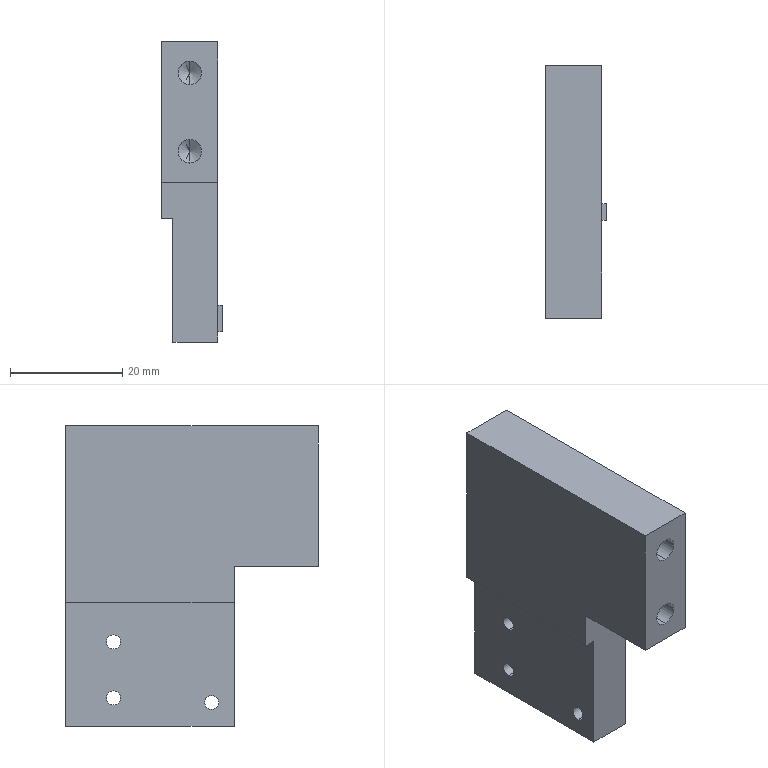Part | SolidWorks | features ICE 4, HoleWzd 3, ExtruThin 1 | 1 solid | 29 faces | box 10.8 x 45 x 53.5 mm | volume 18015 mm3 | plane 15 | cylinder 10 | cone 4 | commonest cylinder face diameters 2.5 x6 4.2 x4
STEP:
#1=CARTESIAN_POINT('',(10.8,19.,-25.55));
#2=VERTEX_POINT('',#1);
#3=CARTESIAN_POINT('',(10.8,19.,-23.05));
#4=VERTEX_POINT('',#3);
#5=CARTESIAN_POINT('',(10.8,19.,-24.3));
#6=DIRECTION('',(-1.,0.,0.));
#7=DIRECTION('',(0.,0.,1.));
#8=AXIS2_PLACEMENT_3D('',#5,#6,#7);
#9=CIRCLE('',#8,1.25);
#10=EDGE_CURVE('',#2,#4,#9,.T.);
#11=ORIENTED_EDGE('',*,*,#10,.F.);
#12=CARTESIAN_POINT('',(2.,19.,-25.55));
#13=VERTEX_POINT('',#12);
#14=CARTESIAN_POINT('',(0.,19.,-25.55));
#15=DIRECTION('',(-1.,0.,0.));
#16=VECTOR('',#15,1000.);
#17=LINE('',#14,#16);
#18=EDGE_CURVE('',#2,#13,#17,.T.);
#19=ORIENTED_EDGE('',*,*,#18,.T.);
#20=CARTESIAN_POINT('',(2.,19.,-23.05));
#21=VERTEX_POINT('',#20);
#22=CARTESIAN_POINT('',(2.,19.,-24.3));
#23=DIRECTION('',(1.,0.,0.));
#24=DIRECTION('',(0.,0.,-1.));
#25=AXIS2_PLACEMENT_3D('',#22,#23,#24);
#26=CIRCLE('',#25,1.25);
#27=EDGE_CURVE('',#21,#13,#26,.T.);
#28=ORIENTED_EDGE('',*,*,#27,.F.);
#29=CARTESIAN_POINT('',(0.,19.,-23.05));
#30=DIRECTION('',(-1.,0.,0.));
#31=VECTOR('',#30,1000.);
#32=LINE('',#29,#31);
#33=EDGE_CURVE('',#4,#21,#32,.T.);
#34=ORIENTED_EDGE('',*,*,#33,.F.);
#35=EDGE_LOOP('',(#11,#19,#28,#34));
#36=FACE_OUTER_BOUND('',#35,.T.);
#37=CARTESIAN_POINT('',(0.,19.,-24.3));
#38=DIRECTION('',(-1.,0.,0.));
#39=DIRECTION('',(0.,0.,1.));
#40=AXIS2_PLACEMENT_3D('',#37,#38,#39);
#41=CYLINDRICAL_SURFACE('',#40,1.25);
#42=ADVANCED_FACE('',(#36),#41,.F.);
#43=CARTESIAN_POINT('',(5.,12.4,7.6));
#44=VERTEX_POINT('',#43);
#45=CARTESIAN_POINT('',(5.,12.4,3.4));
#46=VERTEX_POINT('',#45);
#47=CARTESIAN_POINT('',(5.,12.4,5.5));
#48=DIRECTION('',(0.,-1.,0.));
#49=DIRECTION('',(0.,0.,-1.));
#50=AXIS2_PLACEMENT_3D('',#47,#48,#49);
#51=CIRCLE('',#50,2.1);
#52=EDGE_CURVE('',#44,#46,#51,.T.);
#53=ORIENTED_EDGE('',*,*,#52,.F.);
#54=CARTESIAN_POINT('',(5.,0.,7.6));
#55=VERTEX_POINT('',#54);
#56=CARTESIAN_POINT('',(5.,0.,7.6));
#57=DIRECTION('',(0.,-1.,0.));
#58=VECTOR('',#57,1000.);
#59=LINE('',#56,#58);
#60=EDGE_CURVE('',#44,#55,#59,.T.);
#61=ORIENTED_EDGE('',*,*,#60,.T.);
#62=CARTESIAN_POINT('',(5.,0.,3.4));
#63=VERTEX_POINT('',#62);
#64=CARTESIAN_POINT('',(5.,0.,5.5));
#65=DIRECTION('',(0.,-1.,0.));
#66=DIRECTION('',(0.,0.,-1.));
#67=AXIS2_PLACEMENT_3D('',#64,#65,#66);
#68=CIRCLE('',#67,2.1);
#69=EDGE_CURVE('',#55,#63,#68,.T.);
#70=ORIENTED_EDGE('',*,*,#69,.T.);
#71=CARTESIAN_POINT('',(5.,0.,3.4));
#72=DIRECTION('',(0.,-1.,0.));
#73=VECTOR('',#72,1000.);
#74=LINE('',#71,#73);
#75=EDGE_CURVE('',#46,#63,#74,.T.);
#76=ORIENTED_EDGE('',*,*,#75,.F.);
#77=EDGE_LOOP('',(#53,#61,#70,#76));
#78=FACE_OUTER_BOUND('',#77,.T.);
#79=CARTESIAN_POINT('',(5.,0.,5.5));
#80=DIRECTION('',(0.,-1.,0.));
#81=DIRECTION('',(0.,0.,-1.));
#82=AXIS2_PLACEMENT_3D('',#79,#80,#81);
#83=CYLINDRICAL_SURFACE('',#82,2.1);
#84=ADVANCED_FACE('',(#78),#83,.F.);
#85=CARTESIAN_POINT('',(5.,13.662,5.5));
#86=VERTEX_POINT('',#85);
#87=CARTESIAN_POINT('',(5.,12.4,3.4));
#88=DIRECTION('',(0.,-0.515,-0.8572));
#89=VECTOR('',#88,1000.);
#90=LINE('',#87,#89);
#91=EDGE_CURVE('',#86,#46,#90,.T.);
#92=ORIENTED_EDGE('',*,*,#91,.F.);
#93=CARTESIAN_POINT('',(5.,12.4,7.6));
#94=DIRECTION('',(0.,-0.515,0.8572));
#95=VECTOR('',#94,1000.);
#96=LINE('',#93,#95);
#97=EDGE_CURVE('',#86,#44,#96,.T.);
#98=ORIENTED_EDGE('',*,*,#97,.T.);
#99=ORIENTED_EDGE('',*,*,#52,.T.);
#100=EDGE_LOOP('',(#92,#98,#99));
#101=FACE_OUTER_BOUND('',#100,.T.);
#102=CARTESIAN_POINT('',(5.,12.4,5.5));
#103=DIRECTION('',(0.,-1.,0.));
#104=DIRECTION('',(0.,0.,-1.));
#105=AXIS2_PLACEMENT_3D('',#102,#103,#104);
#106=CONICAL_SURFACE('',#105,2.1,1.03);
#107=ADVANCED_FACE('',(#101),#106,.F.);
#108=CARTESIAN_POINT('',(5.,12.4,21.6));
#109=VERTEX_POINT('',#108);
#110=CARTESIAN_POINT('',(5.,12.4,17.4));
#111=VERTEX_POINT('',#110);
#112=CARTESIAN_POINT('',(5.,12.4,19.5));
#113=DIRECTION('',(0.,-1.,0.));
#114=DIRECTION('',(0.,0.,-1.));
#115=AXIS2_PLACEMENT_3D('',#112,#113,#114);
#116=CIRCLE('',#115,2.1);
#117=EDGE_CURVE('',#109,#111,#116,.T.);
#118=ORIENTED_EDGE('',*,*,#117,.F.);
#119=CARTESIAN_POINT('',(5.,0.,21.6));
#120=VERTEX_POINT('',#119);
#121=CARTESIAN_POINT('',(5.,0.,21.6));
#122=DIRECTION('',(0.,-1.,0.));
#123=VECTOR('',#122,1000.);
#124=LINE('',#121,#123);
#125=EDGE_CURVE('',#109,#120,#124,.T.);
#126=ORIENTED_EDGE('',*,*,#125,.T.);
#127=CARTESIAN_POINT('',(5.,0.,17.4));
#128=VERTEX_POINT('',#127);
#129=CARTESIAN_POINT('',(5.,0.,19.5));
#130=DIRECTION('',(0.,-1.,0.));
#131=DIRECTION('',(0.,0.,-1.));
#132=AXIS2_PLACEMENT_3D('',#129,#130,#131);
#133=CIRCLE('',#132,2.1);
#134=EDGE_CURVE('',#120,#128,#133,.T.);
#135=ORIENTED_EDGE('',*,*,#134,.T.);
#136=CARTESIAN_POINT('',(5.,0.,17.4));
#137=DIRECTION('',(0.,-1.,0.));
#138=VECTOR('',#137,1000.);
#139=LINE('',#136,#138);
#140=EDGE_CURVE('',#111,#128,#139,.T.);
#141=ORIENTED_EDGE('',*,*,#140,.F.);
#142=EDGE_LOOP('',(#118,#126,#135,#141));
#143=FACE_OUTER_BOUND('',#142,.T.);
#144=CARTESIAN_POINT('',(5.,0.,19.5));
#145=DIRECTION('',(0.,-1.,0.));
#146=DIRECTION('',(0.,0.,-1.));
#147=AXIS2_PLACEMENT_3D('',#144,#145,#146);
#148=CYLINDRICAL_SURFACE('',#147,2.1);
#149=ADVANCED_FACE('',(#143),#148,.F.);
#150=CARTESIAN_POINT('',(5.,13.662,19.5));
#151=VERTEX_POINT('',#150);
#152=CARTESIAN_POINT('',(5.,12.4,17.4));
#153=DIRECTION('',(0.,-0.515,-0.8572));
#154=VECTOR('',#153,1000.);
#155=LINE('',#152,#154);
#156=EDGE_CURVE('',#151,#111,#155,.T.);
#157=ORIENTED_EDGE('',*,*,#156,.F.);
#158=CARTESIAN_POINT('',(5.,12.4,21.6));
#159=DIRECTION('',(0.,-0.515,0.8572));
#160=VECTOR('',#159,1000.);
#161=LINE('',#158,#160);
#162=EDGE_CURVE('',#151,#109,#161,.T.);
#163=ORIENTED_EDGE('',*,*,#162,.T.);
#164=ORIENTED_EDGE('',*,*,#117,.T.);
#165=EDGE_LOOP('',(#157,#163,#164));
#166=FACE_OUTER_BOUND('',#165,.T.);
#167=CARTESIAN_POINT('',(5.,12.4,19.5));
#168=DIRECTION('',(0.,-1.,0.));
#169=DIRECTION('',(0.,0.,-1.));
#170=AXIS2_PLACEMENT_3D('',#167,#168,#169);
#171=CONICAL_SURFACE('',#170,2.1,1.03);
#172=ADVANCED_FACE('',(#166),#171,.F.);
#173=CARTESIAN_POINT('',(2.,36.5,-12.25));
#174=VERTEX_POINT('',#173);
#175=CARTESIAN_POINT('',(2.,36.5,-14.75));
#176=VERTEX_POINT('',#175);
#177=CARTESIAN_POINT('',(2.,36.5,-13.5));
#178=DIRECTION('',(1.,0.,0.));
#179=DIRECTION('',(0.,0.,-1.));
#180=AXIS2_PLACEMENT_3D('',#177,#178,#179);
#181=CIRCLE('',#180,1.25);
#182=EDGE_CURVE('',#174,#176,#181,.T.);
#183=ORIENTED_EDGE('',*,*,#182,.F.);
#184=CARTESIAN_POINT('',(10.,36.5,-12.25));
#185=VERTEX_POINT('',#184);
#186=CARTESIAN_POINT('',(10.,36.5,-12.25));
#187=DIRECTION('',(1.,0.,0.));
#188=VECTOR('',#187,1000.);
#189=LINE('',#186,#188);
#190=EDGE_CURVE('',#174,#185,#189,.T.);
#191=ORIENTED_EDGE('',*,*,#190,.T.);
#192=CARTESIAN_POINT('',(10.,36.5,-14.75));
#193=VERTEX_POINT('',#192);
#194=CARTESIAN_POINT('',(10.,36.5,-13.5));
#195=DIRECTION('',(1.,0.,0.));
#196=DIRECTION('',(0.,0.,-1.));
#197=AXIS2_PLACEMENT_3D('',#194,#195,#196);
#198=CIRCLE('',#197,1.25);
#199=EDGE_CURVE('',#185,#193,#198,.T.);
#200=ORIENTED_EDGE('',*,*,#199,.T.);
#201=CARTESIAN_POINT('',(10.,36.5,-14.75));
#202=DIRECTION('',(1.,0.,0.));
#203=VECTOR('',#202,1000.);
#204=LINE('',#201,#203);
#205=EDGE_CURVE('',#176,#193,#204,.T.);
#206=ORIENTED_EDGE('',*,*,#205,.F.);
#207=EDGE_LOOP('',(#183,#191,#200,#206));
#208=FACE_OUTER_BOUND('',#207,.T.);
#209=CARTESIAN_POINT('',(10.,36.5,-13.5));
#210=DIRECTION('',(1.,0.,0.));
#211=DIRECTION('',(0.,0.,-1.));
#212=AXIS2_PLACEMENT_3D('',#209,#210,#211);
#213=CYLINDRICAL_SURFACE('',#212,1.25);
#214=ADVANCED_FACE('',(#208),#213,.F.);
#215=CARTESIAN_POINT('',(2.,36.5,-22.25));
#216=VERTEX_POINT('',#215);
#217=CARTESIAN_POINT('',(2.,36.5,-24.75));
#218=VERTEX_POINT('',#217);
#219=CARTESIAN_POINT('',(2.,36.5,-23.5));
#220=DIRECTION('',(1.,0.,0.));
#221=DIRECTION('',(0.,0.,-1.));
#222=AXIS2_PLACEMENT_3D('',#219,#220,#221);
#223=CIRCLE('',#222,1.25);
#224=EDGE_CURVE('',#216,#218,#223,.T.);
#225=ORIENTED_EDGE('',*,*,#224,.F.);
#226=CARTESIAN_POINT('',(10.,36.5,-22.25));
#227=VERTEX_POINT('',#226);
#228=CARTESIAN_POINT('',(10.,36.5,-22.25));
#229=DIRECTION('',(1.,0.,0.));
#230=VECTOR('',#229,1000.);
#231=LINE('',#228,#230);
#232=EDGE_CURVE('',#216,#227,#231,.T.);
#233=ORIENTED_EDGE('',*,*,#232,.T.);
#234=CARTESIAN_POINT('',(10.,36.5,-24.75));
#235=VERTEX_POINT('',#234);
#236=CARTESIAN_POINT('',(10.,36.5,-23.5));
#237=DIRECTION('',(1.,0.,0.));
#238=DIRECTION('',(0.,0.,-1.));
#239=AXIS2_PLACEMENT_3D('',#236,#237,#238);
#240=CIRCLE('',#239,1.25);
#241=EDGE_CURVE('',#227,#235,#240,.T.);
#242=ORIENTED_EDGE('',*,*,#241,.T.);
#243=CARTESIAN_POINT('',(10.,36.5,-24.75));
#244=DIRECTION('',(1.,0.,0.));
#245=VECTOR('',#244,1000.);
#246=LINE('',#243,#245);
#247=EDGE_CURVE('',#218,#235,#246,.T.);
#248=ORIENTED_EDGE('',*,*,#247,.F.);
#249=EDGE_LOOP('',(#225,#233,#242,#248));
#250=FACE_OUTER_BOUND('',#249,.T.);
#251=CARTESIAN_POINT('',(10.,36.5,-23.5));
#252=DIRECTION('',(1.,0.,0.));
#253=DIRECTION('',(0.,0.,-1.));
#254=AXIS2_PLACEMENT_3D('',#251,#252,#253);
#255=CYLINDRICAL_SURFACE('',#254,1.25);
#256=ADVANCED_FACE('',(#250),#255,.F.);
#257=CARTESIAN_POINT('',(10.,0.,0.));
#258=VERTEX_POINT('',#257);
#259=CARTESIAN_POINT('',(10.,0.,25.));
#260=VERTEX_POINT('',#259);
#261=CARTESIAN_POINT('',(10.,0.,25.));
#262=DIRECTION('',(0.,0.,1.));
#263=VECTOR('',#262,1000.);
#264=LINE('',#261,#263);
#265=EDGE_CURVE('',#258,#260,#264,.T.);
#266=ORIENTED_EDGE('',*,*,#265,.F.);
#267=CARTESIAN_POINT('',(10.,15.,0.));
#268=VERTEX_POINT('',#267);
#269=CARTESIAN_POINT('',(10.,0.,0.));
#270=DIRECTION('',(0.,1.,0.));
#271=VECTOR('',#270,1000.);
#272=LINE('',#269,#271);
#273=EDGE_CURVE('',#258,#268,#272,.T.);
#274=ORIENTED_EDGE('',*,*,#273,.T.);
#275=CARTESIAN_POINT('',(10.,15.,-28.5));
#276=VERTEX_POINT('',#275);
#277=CARTESIAN_POINT('',(10.,15.,0.));
#278=DIRECTION('',(0.,0.,-1.));
#279=VECTOR('',#278,1000.);
#280=LINE('',#277,#279);
#281=EDGE_CURVE('',#268,#276,#280,.T.);
#282=ORIENTED_EDGE('',*,*,#281,.T.);
#283=CARTESIAN_POINT('',(10.,45.,-28.5));
#284=VERTEX_POINT('',#283);
#285=CARTESIAN_POINT('',(10.,45.,-28.5));
#286=DIRECTION('',(0.,1.,0.));
#287=VECTOR('',#286,1000.);
#288=LINE('',#285,#287);
#289=EDGE_CURVE('',#276,#284,#288,.T.);
#290=ORIENTED_EDGE('',*,*,#289,.T.);
#291=CARTESIAN_POINT('',(10.,45.,25.));
#292=VERTEX_POINT('',#291);
#293=CARTESIAN_POINT('',(10.,45.,25.));
#294=DIRECTION('',(0.,0.,-1.));
#295=VECTOR('',#294,1000.);
#296=LINE('',#293,#295);
#297=EDGE_CURVE('',#292,#284,#296,.T.);
#298=ORIENTED_EDGE('',*,*,#297,.F.);
#299=CARTESIAN_POINT('',(10.,0.,25.));
#300=DIRECTION('',(0.,1.,0.));
#301=VECTOR('',#300,1000.);
#302=LINE('',#299,#301);
#303=EDGE_CURVE('',#260,#292,#302,.T.);
#304=ORIENTED_EDGE('',*,*,#303,.F.);
#305=EDGE_LOOP('',(#266,#274,#282,#290,#298,#304));
#306=FACE_OUTER_BOUND('',#305,.T.);
#307=CARTESIAN_POINT('',(10.,36.5,-13.5));
#308=DIRECTION('',(1.,0.,0.));
#309=DIRECTION('',(0.,0.,-1.));
#310=AXIS2_PLACEMENT_3D('',#307,#308,#309);
#311=CIRCLE('',#310,1.25);
#312=EDGE_CURVE('',#193,#185,#311,.T.);
#313=ORIENTED_EDGE('',*,*,#312,.F.);
#314=ORIENTED_EDGE('',*,*,#199,.F.);
#315=EDGE_LOOP('',(#313,#314));
#316=FACE_BOUND('',#315,.T.);
#317=CARTESIAN_POINT('',(10.,36.5,-23.5));
#318=DIRECTION('',(1.,0.,0.));
#319=DIRECTION('',(0.,0.,-1.));
#320=AXIS2_PLACEMENT_3D('',#317,#318,#319);
#321=CIRCLE('',#320,1.25);
#322=EDGE_CURVE('',#235,#227,#321,.T.);
#323=ORIENTED_EDGE('',*,*,#322,.F.);
#324=ORIENTED_EDGE('',*,*,#241,.F.);
#325=EDGE_LOOP('',(#323,#324));
#326=FACE_BOUND('',#325,.T.);
#327=CARTESIAN_POINT('',(10.,17.5,-26.7));
#328=VERTEX_POINT('',#327);
#329=CARTESIAN_POINT('',(10.,20.5,-26.7));
#330=VERTEX_POINT('',#329);
#331=CARTESIAN_POINT('',(10.,20.5,-26.7));
#332=DIRECTION('',(0.,1.,0.));
#333=VECTOR('',#332,1000.);
#334=LINE('',#331,#333);
#335=EDGE_CURVE('',#328,#330,#334,.T.);
#336=ORIENTED_EDGE('',*,*,#335,.F.);
#337=CARTESIAN_POINT('',(10.,17.5,-21.9));
#338=VERTEX_POINT('',#337);
#339=CARTESIAN_POINT('',(10.,17.5,-21.9));
#340=DIRECTION('',(0.,0.,-1.));
#341=VECTOR('',#340,1000.);
#342=LINE('',#339,#341);
#343=EDGE_CURVE('',#338,#328,#342,.T.);
#344=ORIENTED_EDGE('',*,*,#343,.F.);
#345=CARTESIAN_POINT('',(10.,20.5,-21.9));
#346=VERTEX_POINT('',#345);
#347=CARTESIAN_POINT('',(10.,20.5,-21.9));
#348=DIRECTION('',(0.,-1.,0.));
#349=VECTOR('',#348,1000.);
#350=LINE('',#347,#349);
#351=EDGE_CURVE('',#346,#338,#350,.T.);
#352=ORIENTED_EDGE('',*,*,#351,.F.);
#353=CARTESIAN_POINT('',(10.,20.5,-21.9));
#354=DIRECTION('',(0.,0.,1.));
#355=VECTOR('',#354,1000.);
#356=LINE('',#353,#355);
#357=EDGE_CURVE('',#330,#346,#356,.T.);
#358=ORIENTED_EDGE('',*,*,#357,.F.);
#359=EDGE_LOOP('',(#336,#344,#352,#358));
#360=FACE_BOUND('',#359,.T.);
#361=CARTESIAN_POINT('',(10.,0.,25.));
#362=DIRECTION('',(-1.,0.,0.));
#363=DIRECTION('',(0.,0.,1.));
#364=AXIS2_PLACEMENT_3D('',#361,#362,#363);
#365=PLANE('',#364);
#366=ADVANCED_FACE('',(#306,#316,#326,#360),#365,.F.);
#367=CARTESIAN_POINT('',(0.,0.,25.));
#368=VERTEX_POINT('',#367);
#369=CARTESIAN_POINT('',(0.,0.,25.));
#370=DIRECTION('',(-1.,0.,0.));
#371=VECTOR('',#370,1000.);
#372=LINE('',#369,#371);
#373=EDGE_CURVE('',#260,#368,#372,.T.);
#374=ORIENTED_EDGE('',*,*,#373,.F.);
#375=ORIENTED_EDGE('',*,*,#303,.T.);
#376=CARTESIAN_POINT('',(0.,45.,25.));
#377=VERTEX_POINT('',#376);
#378=CARTESIAN_POINT('',(0.,45.,25.));
#379=DIRECTION('',(1.,0.,0.));
#380=VECTOR('',#379,1000.);
#381=LINE('',#378,#380);
#382=EDGE_CURVE('',#377,#292,#381,.T.);
#383=ORIENTED_EDGE('',*,*,#382,.F.);
#384=CARTESIAN_POINT('',(0.,0.,25.));
#385=DIRECTION('',(0.,1.,0.));
#386=VECTOR('',#385,1000.);
#387=LINE('',#384,#386);
#388=EDGE_CURVE('',#368,#377,#387,.T.);
#389=ORIENTED_EDGE('',*,*,#388,.F.);
#390=EDGE_LOOP('',(#374,#375,#383,#389));
#391=FACE_OUTER_BOUND('',#390,.T.);
#392=CARTESIAN_POINT('',(0.,0.,25.));
#393=DIRECTION('',(0.,0.,-1.));
#394=DIRECTION('',(-1.,0.,0.));
#395=AXIS2_PLACEMENT_3D('',#392,#393,#394);
#396=PLANE('',#395);
#397=ADVANCED_FACE('',(#391),#396,.F.);
#398=ORIENTED_EDGE('',*,*,#273,.F.);
#399=CARTESIAN_POINT('',(0.,0.,0.));
#400=VERTEX_POINT('',#399);
#401=CARTESIAN_POINT('',(0.,0.,0.));
#402=DIRECTION('',(-1.,0.,0.));
#403=VECTOR('',#402,1000.);
#404=LINE('',#401,#403);
#405=EDGE_CURVE('',#258,#400,#404,.T.);
#406=ORIENTED_EDGE('',*,*,#405,.T.);
#407=CARTESIAN_POINT('',(0.,15.,0.));
#408=VERTEX_POINT('',#407);
#409=CARTESIAN_POINT('',(0.,0.,0.));
#410=DIRECTION('',(0.,1.,0.));
#411=VECTOR('',#410,1000.);
#412=LINE('',#409,#411);
#413=EDGE_CURVE('',#400,#408,#412,.T.);
#414=ORIENTED_EDGE('',*,*,#413,.T.);
#415=CARTESIAN_POINT('',(51.379,15.,0.));
#416=DIRECTION('',(-1.,0.,0.));
#417=VECTOR('',#416,1000.);
#418=LINE('',#415,#417);
#419=EDGE_CURVE('',#268,#408,#418,.T.);
#420=ORIENTED_EDGE('',*,*,#419,.F.);
#421=EDGE_LOOP('',(#398,#406,#414,#420));
#422=FACE_OUTER_BOUND('',#421,.T.);
#423=CARTESIAN_POINT('',(0.,0.,0.));
#424=DIRECTION('',(0.,0.,-1.));
#425=DIRECTION('',(-1.,0.,0.));
#426=AXIS2_PLACEMENT_3D('',#423,#424,#425);
#427=PLANE('',#426);
#428=ADVANCED_FACE('',(#422),#427,.T.);
#429=CARTESIAN_POINT('',(2.,45.,-6.5));
#430=VERTEX_POINT('',#429);
#431=CARTESIAN_POINT('',(2.,45.,-28.5));
#432=VERTEX_POINT('',#431);
#433=CARTESIAN_POINT('',(2.,45.,-28.5));
#434=DIRECTION('',(0.,0.,-1.));
#435=VECTOR('',#434,1000.);
#436=LINE('',#433,#435);
#437=EDGE_CURVE('',#430,#432,#436,.T.);
#438=ORIENTED_EDGE('',*,*,#437,.F.);
#439=CARTESIAN_POINT('',(0.,45.,-6.5));
#440=VERTEX_POINT('',#439);
#441=CARTESIAN_POINT('',(0.,45.,-6.5));
#442=DIRECTION('',(1.,0.,0.));
#443=VECTOR('',#442,1000.);
#444=LINE('',#441,#443);
#445=EDGE_CURVE('',#440,#430,#444,.T.);
#446=ORIENTED_EDGE('',*,*,#445,.F.);
#447=CARTESIAN_POINT('',(0.,45.,25.));
#448=DIRECTION('',(0.,0.,-1.));
#449=VECTOR('',#448,1000.);
#450=LINE('',#447,#449);
#451=EDGE_CURVE('',#377,#440,#450,.T.);
#452=ORIENTED_EDGE('',*,*,#451,.F.);
#453=ORIENTED_EDGE('',*,*,#382,.T.);
#454=ORIENTED_EDGE('',*,*,#297,.T.);
#455=CARTESIAN_POINT('',(51.379,45.,-28.5));
#456=DIRECTION('',(-1.,0.,0.));
#457=VECTOR('',#456,1000.);
#458=LINE('',#455,#457);
#459=EDGE_CURVE('',#284,#432,#458,.T.);
#460=ORIENTED_EDGE('',*,*,#459,.T.);
#461=EDGE_LOOP('',(#438,#446,#452,#453,#454,#460));
#462=FACE_OUTER_BOUND('',#461,.T.);
#463=CARTESIAN_POINT('',(0.,45.,25.));
#464=DIRECTION('',(0.,1.,0.));
#465=DIRECTION('',(0.,0.,1.));
#466=AXIS2_PLACEMENT_3D('',#463,#464,#465);
#467=PLANE('',#466);
#468=ADVANCED_FACE('',(#462),#467,.T.);
#469=CARTESIAN_POINT('',(0.,15.,-6.5));
#470=VERTEX_POINT('',#469);
#471=CARTESIAN_POINT('',(0.,-10.,-6.5));
#472=DIRECTION('',(0.,1.,0.));
#473=VECTOR('',#472,1000.);
#474=LINE('',#471,#473);
#475=EDGE_CURVE('',#470,#440,#474,.T.);
#476=ORIENTED_EDGE('',*,*,#475,.F.);
#477=CARTESIAN_POINT('',(0.,15.,0.));
#478=DIRECTION('',(0.,0.,1.));
#479=VECTOR('',#478,1000.);
#480=LINE('',#477,#479);
#481=EDGE_CURVE('',#470,#408,#480,.T.);
#482=ORIENTED_EDGE('',*,*,#481,.T.);
#483=ORIENTED_EDGE('',*,*,#413,.F.);
#484=CARTESIAN_POINT('',(0.,0.,25.));
#485=DIRECTION('',(0.,0.,-1.));
#486=VECTOR('',#485,1000.);
#487=LINE('',#484,#486);
#488=EDGE_CURVE('',#368,#400,#487,.T.);
#489=ORIENTED_EDGE('',*,*,#488,.F.);
#490=ORIENTED_EDGE('',*,*,#388,.T.);
#491=ORIENTED_EDGE('',*,*,#451,.T.);
#492=EDGE_LOOP('',(#476,#482,#483,#489,#490,#491));
#493=FACE_OUTER_BOUND('',#492,.T.);
#494=CARTESIAN_POINT('',(0.,0.,25.));
#495=DIRECTION('',(-1.,0.,0.));
#496=DIRECTION('',(0.,0.,1.));
#497=AXIS2_PLACEMENT_3D('',#494,#495,#496);
#498=PLANE('',#497);
#499=ADVANCED_FACE('',(#493),#498,.T.);
#500=CARTESIAN_POINT('',(2.,15.,-28.5));
#501=VERTEX_POINT('',#500);
#502=CARTESIAN_POINT('',(2.,15.,-6.5));
#503=VERTEX_POINT('',#502);
#504=CARTESIAN_POINT('',(2.,15.,0.));
#505=DIRECTION('',(0.,0.,1.));
#506=VECTOR('',#505,1000.);
#507=LINE('',#504,#506);
#508=EDGE_CURVE('',#501,#503,#507,.T.);
#509=ORIENTED_EDGE('',*,*,#508,.F.);
#510=CARTESIAN_POINT('',(51.379,15.,-28.5));
#511=DIRECTION('',(-1.,0.,0.));
#512=VECTOR('',#511,1000.);
#513=LINE('',#510,#512);
#514=EDGE_CURVE('',#276,#501,#513,.T.);
#515=ORIENTED_EDGE('',*,*,#514,.F.);
#516=ORIENTED_EDGE('',*,*,#281,.F.);
#517=ORIENTED_EDGE('',*,*,#419,.T.);
#518=ORIENTED_EDGE('',*,*,#481,.F.);
#519=CARTESIAN_POINT('',(51.379,15.,-6.5));
#520=DIRECTION('',(-1.,0.,0.));
#521=VECTOR('',#520,1000.);
#522=LINE('',#519,#521);
#523=EDGE_CURVE('',#503,#470,#522,.T.);
#524=ORIENTED_EDGE('',*,*,#523,.F.);
#525=EDGE_LOOP('',(#509,#515,#516,#517,#518,#524));
#526=FACE_OUTER_BOUND('',#525,.T.);
#527=CARTESIAN_POINT('',(51.379,15.,0.));
#528=DIRECTION('',(0.,-1.,0.));
#529=DIRECTION('',(0.,0.,-1.));
#530=AXIS2_PLACEMENT_3D('',#527,#528,#529);
#531=PLANE('',#530);
#532=ADVANCED_FACE('',(#526),#531,.T.);
#533=CARTESIAN_POINT('',(2.,45.,-28.5));
#534=DIRECTION('',(0.,-1.,0.));
#535=VECTOR('',#534,1000.);
#536=LINE('',#533,#535);
#537=EDGE_CURVE('',#432,#501,#536,.T.);
#538=ORIENTED_EDGE('',*,*,#537,.F.);
#539=ORIENTED_EDGE('',*,*,#459,.F.);
#540=ORIENTED_EDGE('',*,*,#289,.F.);
#541=ORIENTED_EDGE('',*,*,#514,.T.);
#542=EDGE_LOOP('',(#538,#539,#540,#541));
#543=FACE_OUTER_BOUND('',#542,.T.);
#544=CARTESIAN_POINT('',(51.379,45.,-28.5));
#545=DIRECTION('',(0.,0.,-1.));
#546=DIRECTION('',(0.,1.,0.));
#547=AXIS2_PLACEMENT_3D('',#544,#545,#546);
#548=PLANE('',#547);
#549=ADVANCED_FACE('',(#543),#548,.T.);
#550=ORIENTED_EDGE('',*,*,#27,.T.);
#551=CARTESIAN_POINT('',(2.,19.,-24.3));
#552=DIRECTION('',(1.,0.,0.));
#553=DIRECTION('',(0.,0.,-1.));
#554=AXIS2_PLACEMENT_3D('',#551,#552,#553);
#555=CIRCLE('',#554,1.25);
#556=EDGE_CURVE('',#13,#21,#555,.T.);
#557=ORIENTED_EDGE('',*,*,#556,.T.);
#558=EDGE_LOOP('',(#550,#557));
#559=FACE_BOUND('',#558,.T.);
#560=CARTESIAN_POINT('',(2.,36.5,-13.5));
#561=DIRECTION('',(1.,0.,0.));
#562=DIRECTION('',(0.,0.,-1.));
#563=AXIS2_PLACEMENT_3D('',#560,#561,#562);
#564=CIRCLE('',#563,1.25);
#565=EDGE_CURVE('',#176,#174,#564,.T.);
#566=ORIENTED_EDGE('',*,*,#565,.T.);
#567=ORIENTED_EDGE('',*,*,#182,.T.);
#568=EDGE_LOOP('',(#566,#567));
#569=FACE_BOUND('',#568,.T.);
#570=CARTESIAN_POINT('',(2.,36.5,-23.5));
#571=DIRECTION('',(1.,0.,0.));
#572=DIRECTION('',(0.,0.,-1.));
#573=AXIS2_PLACEMENT_3D('',#570,#571,#572);
#574=CIRCLE('',#573,1.25);
#575=EDGE_CURVE('',#218,#216,#574,.T.);
#576=ORIENTED_EDGE('',*,*,#575,.T.);
#577=ORIENTED_EDGE('',*,*,#224,.T.);
#578=EDGE_LOOP('',(#576,#577));
#579=FACE_BOUND('',#578,.T.);
#580=ORIENTED_EDGE('',*,*,#508,.T.);
#581=CARTESIAN_POINT('',(2.,-10.,-6.5));
#582=DIRECTION('',(0.,1.,0.));
#583=VECTOR('',#582,1000.);
#584=LINE('',#581,#583);
#585=EDGE_CURVE('',#503,#430,#584,.T.);
#586=ORIENTED_EDGE('',*,*,#585,.T.);
#587=ORIENTED_EDGE('',*,*,#437,.T.);
#588=ORIENTED_EDGE('',*,*,#537,.T.);
#589=EDGE_LOOP('',(#580,#586,#587,#588));
#590=FACE_OUTER_BOUND('',#589,.T.);
#591=CARTESIAN_POINT('',(2.,-10.,-28.5));
#592=DIRECTION('',(1.,0.,0.));
#593=DIRECTION('',(0.,0.,-1.));
#594=AXIS2_PLACEMENT_3D('',#591,#592,#593);
#595=PLANE('',#594);
#596=ADVANCED_FACE('',(#559,#569,#579,#590),#595,.F.);
#597=ORIENTED_EDGE('',*,*,#523,.T.);
#598=ORIENTED_EDGE('',*,*,#475,.T.);
#599=ORIENTED_EDGE('',*,*,#445,.T.);
#600=ORIENTED_EDGE('',*,*,#585,.F.);
#601=EDGE_LOOP('',(#597,#598,#599,#600));
#602=FACE_OUTER_BOUND('',#601,.T.);
#603=CARTESIAN_POINT('',(0.,-10.,-6.5));
#604=DIRECTION('',(0.,0.,1.));
#605=DIRECTION('',(1.,0.,0.));
#606=AXIS2_PLACEMENT_3D('',#603,#604,#605);
#607=PLANE('',#606);
#608=ADVANCED_FACE('',(#602),#607,.F.);
#609=ORIENTED_EDGE('',*,*,#232,.F.);
#610=ORIENTED_EDGE('',*,*,#575,.F.);
#611=ORIENTED_EDGE('',*,*,#247,.T.);
#612=ORIENTED_EDGE('',*,*,#322,.T.);
#613=EDGE_LOOP('',(#609,#610,#611,#612));
#614=FACE_OUTER_BOUND('',#613,.T.);
#615=CARTESIAN_POINT('',(10.,36.5,-23.5));
#616=DIRECTION('',(1.,0.,0.));
#617=DIRECTION('',(0.,0.,-1.));
#618=AXIS2_PLACEMENT_3D('',#615,#616,#617);
#619=CYLINDRICAL_SURFACE('',#618,1.25);
#620=ADVANCED_FACE('',(#614),#619,.F.);
#621=ORIENTED_EDGE('',*,*,#190,.F.);
#622=ORIENTED_EDGE('',*,*,#565,.F.);
#623=ORIENTED_EDGE('',*,*,#205,.T.);
#624=ORIENTED_EDGE('',*,*,#312,.T.);
#625=EDGE_LOOP('',(#621,#622,#623,#624));
#626=FACE_OUTER_BOUND('',#625,.T.);
#627=CARTESIAN_POINT('',(10.,36.5,-13.5));
#628=DIRECTION('',(1.,0.,0.));
#629=DIRECTION('',(0.,0.,-1.));
#630=AXIS2_PLACEMENT_3D('',#627,#628,#629);
#631=CYLINDRICAL_SURFACE('',#630,1.25);
#632=ADVANCED_FACE('',(#626),#631,.F.);
#633=CARTESIAN_POINT('',(5.,0.,5.5));
#634=DIRECTION('',(0.,-1.,0.));
#635=DIRECTION('',(0.,0.,-1.));
#636=AXIS2_PLACEMENT_3D('',#633,#634,#635);
#637=CIRCLE('',#636,2.1);
#638=EDGE_CURVE('',#63,#55,#637,.T.);
#639=ORIENTED_EDGE('',*,*,#638,.F.);
#640=ORIENTED_EDGE('',*,*,#69,.F.);
#641=EDGE_LOOP('',(#639,#640));
#642=FACE_BOUND('',#641,.T.);
#643=CARTESIAN_POINT('',(5.,0.,19.5));
#644=DIRECTION('',(0.,-1.,0.));
#645=DIRECTION('',(0.,0.,-1.));
#646=AXIS2_PLACEMENT_3D('',#643,#644,#645);
#647=CIRCLE('',#646,2.1);
#648=EDGE_CURVE('',#128,#120,#647,.T.);
#649=ORIENTED_EDGE('',*,*,#648,.F.);
#650=ORIENTED_EDGE('',*,*,#134,.F.);
#651=EDGE_LOOP('',(#649,#650));
#652=FACE_BOUND('',#651,.T.);
#653=ORIENTED_EDGE('',*,*,#405,.F.);
#654=ORIENTED_EDGE('',*,*,#265,.T.);
#655=ORIENTED_EDGE('',*,*,#373,.T.);
#656=ORIENTED_EDGE('',*,*,#488,.T.);
#657=EDGE_LOOP('',(#653,#654,#655,#656));
#658=FACE_OUTER_BOUND('',#657,.T.);
#659=CARTESIAN_POINT('',(0.,0.,0.));
#660=DIRECTION('',(0.,-1.,0.));
#661=DIRECTION('',(0.,0.,-1.));
#662=AXIS2_PLACEMENT_3D('',#659,#660,#661);
#663=PLANE('',#662);
#664=ADVANCED_FACE('',(#642,#652,#658),#663,.T.);
#665=ORIENTED_EDGE('',*,*,#162,.F.);
#666=ORIENTED_EDGE('',*,*,#156,.T.);
#667=CARTESIAN_POINT('',(5.,12.4,19.5));
#668=DIRECTION('',(0.,-1.,0.));
#669=DIRECTION('',(0.,0.,-1.));
#670=AXIS2_PLACEMENT_3D('',#667,#668,#669);
#671=CIRCLE('',#670,2.1);
#672=EDGE_CURVE('',#111,#109,#671,.T.);
#673=ORIENTED_EDGE('',*,*,#672,.T.);
#674=EDGE_LOOP('',(#665,#666,#673));
#675=FACE_OUTER_BOUND('',#674,.T.);
#676=CARTESIAN_POINT('',(5.,12.4,19.5));
#677=DIRECTION('',(0.,-1.,0.));
#678=DIRECTION('',(0.,0.,-1.));
#679=AXIS2_PLACEMENT_3D('',#676,#677,#678);
#680=CONICAL_SURFACE('',#679,2.1,1.03);
#681=ADVANCED_FACE('',(#675),#680,.F.);
#682=ORIENTED_EDGE('',*,*,#125,.F.);
#683=ORIENTED_EDGE('',*,*,#672,.F.);
#684=ORIENTED_EDGE('',*,*,#140,.T.);
#685=ORIENTED_EDGE('',*,*,#648,.T.);
#686=EDGE_LOOP('',(#682,#683,#684,#685));
#687=FACE_OUTER_BOUND('',#686,.T.);
#688=CARTESIAN_POINT('',(5.,0.,19.5));
#689=DIRECTION('',(0.,-1.,0.));
#690=DIRECTION('',(0.,0.,-1.));
#691=AXIS2_PLACEMENT_3D('',#688,#689,#690);
#692=CYLINDRICAL_SURFACE('',#691,2.1);
#693=ADVANCED_FACE('',(#687),#692,.F.);
#694=ORIENTED_EDGE('',*,*,#97,.F.);
#695=ORIENTED_EDGE('',*,*,#91,.T.);
#696=CARTESIAN_POINT('',(5.,12.4,5.5));
#697=DIRECTION('',(0.,-1.,0.));
#698=DIRECTION('',(0.,0.,-1.));
#699=AXIS2_PLACEMENT_3D('',#696,#697,#698);
#700=CIRCLE('',#699,2.1);
#701=EDGE_CURVE('',#46,#44,#700,.T.);
#702=ORIENTED_EDGE('',*,*,#701,.T.);
#703=EDGE_LOOP('',(#694,#695,#702));
#704=FACE_OUTER_BOUND('',#703,.T.);
#705=CARTESIAN_POINT('',(5.,12.4,5.5));
#706=DIRECTION('',(0.,-1.,0.));
#707=DIRECTION('',(0.,0.,-1.));
#708=AXIS2_PLACEMENT_3D('',#705,#706,#707);
#709=CONICAL_SURFACE('',#708,2.1,1.03);
#710=ADVANCED_FACE('',(#704),#709,.F.);
#711=ORIENTED_EDGE('',*,*,#60,.F.);
#712=ORIENTED_EDGE('',*,*,#701,.F.);
#713=ORIENTED_EDGE('',*,*,#75,.T.);
#714=ORIENTED_EDGE('',*,*,#638,.T.);
#715=EDGE_LOOP('',(#711,#712,#713,#714));
#716=FACE_OUTER_BOUND('',#715,.T.);
#717=CARTESIAN_POINT('',(5.,0.,5.5));
#718=DIRECTION('',(0.,-1.,0.));
#719=DIRECTION('',(0.,0.,-1.));
#720=AXIS2_PLACEMENT_3D('',#717,#718,#719);
#721=CYLINDRICAL_SURFACE('',#720,2.1);
#722=ADVANCED_FACE('',(#716),#721,.F.);
#723=ORIENTED_EDGE('',*,*,#335,.T.);
#724=CARTESIAN_POINT('',(10.8,20.5,-26.7));
#725=VERTEX_POINT('',#724);
#726=CARTESIAN_POINT('',(10.8,20.5,-26.7));
#727=DIRECTION('',(-1.,0.,0.));
#728=VECTOR('',#727,1000.);
#729=LINE('',#726,#728);
#730=EDGE_CURVE('',#725,#330,#729,.T.);
#731=ORIENTED_EDGE('',*,*,#730,.F.);
#732=CARTESIAN_POINT('',(10.8,17.5,-26.7));
#733=VERTEX_POINT('',#732);
#734=CARTESIAN_POINT('',(10.8,20.5,-26.7));
#735=DIRECTION('',(0.,1.,0.));
#736=VECTOR('',#735,1000.);
#737=LINE('',#734,#736);
#738=EDGE_CURVE('',#733,#725,#737,.T.);
#739=ORIENTED_EDGE('',*,*,#738,.F.);
#740=CARTESIAN_POINT('',(10.8,17.5,-26.7));
#741=DIRECTION('',(-1.,0.,0.));
#742=VECTOR('',#741,1000.);
#743=LINE('',#740,#742);
#744=EDGE_CURVE('',#733,#328,#743,.T.);
#745=ORIENTED_EDGE('',*,*,#744,.T.);
#746=EDGE_LOOP('',(#723,#731,#739,#745));
#747=FACE_OUTER_BOUND('',#746,.T.);
#748=CARTESIAN_POINT('',(10.8,20.5,-26.7));
#749=DIRECTION('',(0.,0.,1.));
#750=DIRECTION('',(1.,0.,0.));
#751=AXIS2_PLACEMENT_3D('',#748,#749,#750);
#752=PLANE('',#751);
#753=ADVANCED_FACE('',(#747),#752,.F.);
#754=ORIENTED_EDGE('',*,*,#357,.T.);
#755=CARTESIAN_POINT('',(10.8,20.5,-21.9));
#756=VERTEX_POINT('',#755);
#757=CARTESIAN_POINT('',(10.8,20.5,-21.9));
#758=DIRECTION('',(-1.,0.,0.));
#759=VECTOR('',#758,1000.);
#760=LINE('',#757,#759);
#761=EDGE_CURVE('',#756,#346,#760,.T.);
#762=ORIENTED_EDGE('',*,*,#761,.F.);
#763=CARTESIAN_POINT('',(10.8,20.5,-21.9));
#764=DIRECTION('',(0.,0.,1.));
#765=VECTOR('',#764,1000.);
#766=LINE('',#763,#765);
#767=EDGE_CURVE('',#725,#756,#766,.T.);
#768=ORIENTED_EDGE('',*,*,#767,.F.);
#769=ORIENTED_EDGE('',*,*,#730,.T.);
#770=EDGE_LOOP('',(#754,#762,#768,#769));
#771=FACE_OUTER_BOUND('',#770,.T.);
#772=CARTESIAN_POINT('',(10.8,20.5,-21.9));
#773=DIRECTION('',(0.,-1.,0.));
#774=DIRECTION('',(0.,0.,-1.));
#775=AXIS2_PLACEMENT_3D('',#772,#773,#774);
#776=PLANE('',#775);
#777=ADVANCED_FACE('',(#771),#776,.F.);
#778=ORIENTED_EDGE('',*,*,#351,.T.);
#779=CARTESIAN_POINT('',(10.8,17.5,-21.9));
#780=VERTEX_POINT('',#779);
#781=CARTESIAN_POINT('',(10.8,17.5,-21.9));
#782=DIRECTION('',(-1.,0.,0.));
#783=VECTOR('',#782,1000.);
#784=LINE('',#781,#783);
#785=EDGE_CURVE('',#780,#338,#784,.T.);
#786=ORIENTED_EDGE('',*,*,#785,.F.);
#787=CARTESIAN_POINT('',(10.8,20.5,-21.9));
#788=DIRECTION('',(0.,-1.,0.));
#789=VECTOR('',#788,1000.);
#790=LINE('',#787,#789);
#791=EDGE_CURVE('',#756,#780,#790,.T.);
#792=ORIENTED_EDGE('',*,*,#791,.F.);
#793=ORIENTED_EDGE('',*,*,#761,.T.);
#794=EDGE_LOOP('',(#778,#786,#792,#793));
#795=FACE_OUTER_BOUND('',#794,.T.);
#796=CARTESIAN_POINT('',(10.8,20.5,-21.9));
#797=DIRECTION('',(0.,0.,-1.));
#798=DIRECTION('',(-1.,0.,0.));
#799=AXIS2_PLACEMENT_3D('',#796,#797,#798);
#800=PLANE('',#799);
#801=ADVANCED_FACE('',(#795),#800,.F.);
#802=ORIENTED_EDGE('',*,*,#343,.T.);
#803=ORIENTED_EDGE('',*,*,#744,.F.);
#804=CARTESIAN_POINT('',(10.8,17.5,-21.9));
#805=DIRECTION('',(0.,0.,-1.));
#806=VECTOR('',#805,1000.);
#807=LINE('',#804,#806);
#808=EDGE_CURVE('',#780,#733,#807,.T.);
#809=ORIENTED_EDGE('',*,*,#808,.F.);
#810=ORIENTED_EDGE('',*,*,#785,.T.);
#811=EDGE_LOOP('',(#802,#803,#809,#810));
#812=FACE_OUTER_BOUND('',#811,.T.);
#813=CARTESIAN_POINT('',(10.8,17.5,-21.9));
#814=DIRECTION('',(0.,1.,0.));
#815=DIRECTION('',(0.,0.,1.));
#816=AXIS2_PLACEMENT_3D('',#813,#814,#815);
#817=PLANE('',#816);
#818=ADVANCED_FACE('',(#812),#817,.F.);
#819=CARTESIAN_POINT('',(10.8,19.,-24.3));
#820=DIRECTION('',(-1.,0.,0.));
#821=DIRECTION('',(0.,0.,1.));
#822=AXIS2_PLACEMENT_3D('',#819,#820,#821);
#823=CIRCLE('',#822,1.25);
#824=EDGE_CURVE('',#4,#2,#823,.T.);
#825=ORIENTED_EDGE('',*,*,#824,.T.);
#826=ORIENTED_EDGE('',*,*,#10,.T.);
#827=EDGE_LOOP('',(#825,#826));
#828=FACE_BOUND('',#827,.T.);
#829=ORIENTED_EDGE('',*,*,#738,.T.);
#830=ORIENTED_EDGE('',*,*,#767,.T.);
#831=ORIENTED_EDGE('',*,*,#791,.T.);
#832=ORIENTED_EDGE('',*,*,#808,.T.);
#833=EDGE_LOOP('',(#829,#830,#831,#832));
#834=FACE_OUTER_BOUND('',#833,.T.);
#835=CARTESIAN_POINT('',(10.8,0.,0.));
#836=DIRECTION('',(1.,0.,0.));
#837=DIRECTION('',(0.,0.,-1.));
#838=AXIS2_PLACEMENT_3D('',#835,#836,#837);
#839=PLANE('',#838);
#840=ADVANCED_FACE('',(#828,#834),#839,.T.);
#841=ORIENTED_EDGE('',*,*,#18,.F.);
#842=ORIENTED_EDGE('',*,*,#824,.F.);
#843=ORIENTED_EDGE('',*,*,#33,.T.);
#844=ORIENTED_EDGE('',*,*,#556,.F.);
#845=EDGE_LOOP('',(#841,#842,#843,#844));
#846=FACE_OUTER_BOUND('',#845,.T.);
#847=CARTESIAN_POINT('',(0.,19.,-24.3));
#848=DIRECTION('',(-1.,0.,0.));
#849=DIRECTION('',(0.,0.,1.));
#850=AXIS2_PLACEMENT_3D('',#847,#848,#849);
#851=CYLINDRICAL_SURFACE('',#850,1.25);
#852=ADVANCED_FACE('',(#846),#851,.F.);
#853=CLOSED_SHELL('',(#42,#84,#107,#149,#172,#214,#256,#366,#397,#428,#468,#499,#532,#549,#596,#608,#620,#632,#664,#681,#693,#710,#722,#753,#777,#801,#818,#840,#852));
#854=MANIFOLD_SOLID_BREP('',#853);
#855=CARTESIAN_POINT('',(0.,0.,0.));
#856=DIRECTION('',(0.,0.,1.));
#857=DIRECTION('',(1.,0.,0.));
#858=AXIS2_PLACEMENT_3D('',#855,#856,#857);
#859=(LENGTH_UNIT()NAMED_UNIT(*)SI_UNIT(.MILLI.,.METRE.));
#860=UNCERTAINTY_MEASURE_WITH_UNIT(LENGTH_MEASURE(0.00001),#859,'','');
#861=(NAMED_UNIT(*)PLANE_ANGLE_UNIT()SI_UNIT($,.RADIAN.));
#862=(NAMED_UNIT(*)SI_UNIT($,.STERADIAN.)SOLID_ANGLE_UNIT());
#863=(GEOMETRIC_REPRESENTATION_CONTEXT(3)GLOBAL_UNCERTAINTY_ASSIGNED_CONTEXT((#860))GLOBAL_UNIT_ASSIGNED_CONTEXT((#859,#861,#862))REPRESENTATION_CONTEXT('',''));
#864=ADVANCED_BREP_SHAPE_REPRESENTATION('',(#854,#858),#863);